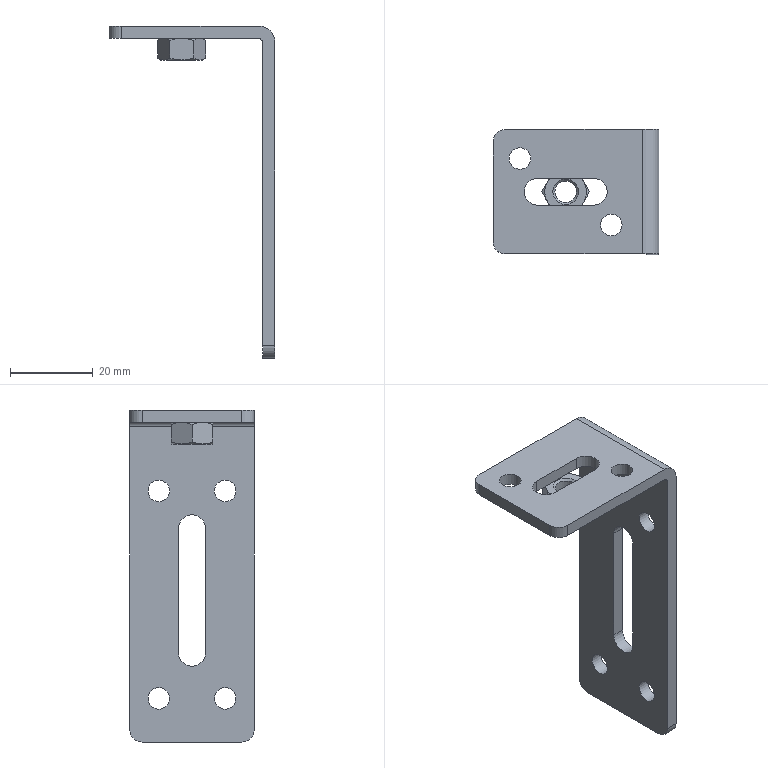Part | STEP file | 冲床-300配套压波_id582_x_t | 1 solid | 51 faces | box 40 x 30 x 80 mm | volume 9315 mm3 | plane 20 | cylinder 17 | cone 14 | commonest cylinder face diameters 5.2 x6 6 x4 6.5 x4 2 x1 5.188 x1 8 x1